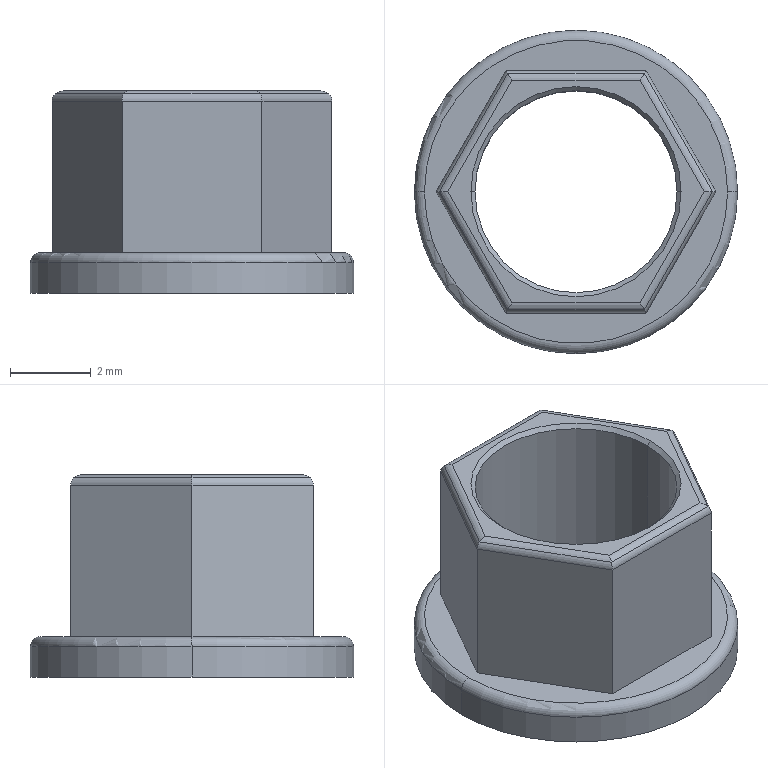Part | SolidWorks | features BaseBody 1 | 1 solid | 29 faces | box 8 x 8 x 5 mm | volume 76.113 mm3 | cylinder 16 | plane 9 | cone 2 | torus 2 | commonest cylinder face diameters 0.5 x12 5 x2 8 x2
STEP:
#1=CARTESIAN_POINT('',(-2.5,0.,4.9));
#2=VERTEX_POINT('',#1);
#3=CARTESIAN_POINT('',(2.5,0.,4.9));
#4=VERTEX_POINT('',#3);
#5=CARTESIAN_POINT('',(0.,0.,4.9));
#6=DIRECTION('',(0.,0.,-1.));
#7=DIRECTION('',(-1.,0.,0.));
#8=AXIS2_PLACEMENT_3D('',#5,#6,#7);
#9=CIRCLE('',#8,2.5);
#10=EDGE_CURVE('',#2,#4,#9,.T.);
#11=ORIENTED_EDGE('',*,*,#10,.T.);
#12=CARTESIAN_POINT('',(2.6,0.,5.));
#13=VERTEX_POINT('',#12);
#14=CARTESIAN_POINT('',(2.55,0.,4.95));
#15=DIRECTION('',(0.7071,0.,0.7071));
#16=VECTOR('',#15,1000.);
#17=LINE('',#14,#16);
#18=EDGE_CURVE('',#4,#13,#17,.T.);
#19=ORIENTED_EDGE('',*,*,#18,.T.);
#20=CARTESIAN_POINT('',(-2.6,0.,5.));
#21=VERTEX_POINT('',#20);
#22=CARTESIAN_POINT('',(0.,0.,5.));
#23=DIRECTION('',(0.,0.,1.));
#24=DIRECTION('',(-1.,0.,0.));
#25=AXIS2_PLACEMENT_3D('',#22,#23,#24);
#26=CIRCLE('',#25,2.6);
#27=EDGE_CURVE('',#13,#21,#26,.T.);
#28=ORIENTED_EDGE('',*,*,#27,.T.);
#29=CARTESIAN_POINT('',(-2.55,0.,4.95));
#30=DIRECTION('',(-0.7071,0.,0.7071));
#31=VECTOR('',#30,1000.);
#32=LINE('',#29,#31);
#33=EDGE_CURVE('',#2,#21,#32,.T.);
#34=ORIENTED_EDGE('',*,*,#33,.F.);
#35=EDGE_LOOP('',(#11,#19,#28,#34));
#36=FACE_OUTER_BOUND('',#35,.T.);
#37=CARTESIAN_POINT('',(0.,0.,4.95));
#38=DIRECTION('',(0.,0.,1.));
#39=DIRECTION('',(-1.,0.,0.));
#40=AXIS2_PLACEMENT_3D('',#37,#38,#39);
#41=CONICAL_SURFACE('',#40,2.55,0.7854);
#42=ADVANCED_FACE('',(#36),#41,.F.);
#43=CARTESIAN_POINT('',(2.5,0.,0.));
#44=VERTEX_POINT('',#43);
#45=CARTESIAN_POINT('',(-2.5,0.,0.));
#46=VERTEX_POINT('',#45);
#47=CARTESIAN_POINT('',(0.,0.,0.));
#48=DIRECTION('',(0.,0.,1.));
#49=DIRECTION('',(-1.,0.,0.));
#50=AXIS2_PLACEMENT_3D('',#47,#48,#49);
#51=CIRCLE('',#50,2.5);
#52=EDGE_CURVE('',#44,#46,#51,.T.);
#53=ORIENTED_EDGE('',*,*,#52,.F.);
#54=CARTESIAN_POINT('',(2.5,0.,5.));
#55=DIRECTION('',(0.,0.,1.));
#56=VECTOR('',#55,1000.);
#57=LINE('',#54,#56);
#58=EDGE_CURVE('',#44,#4,#57,.T.);
#59=ORIENTED_EDGE('',*,*,#58,.T.);
#60=ORIENTED_EDGE('',*,*,#10,.F.);
#61=CARTESIAN_POINT('',(-2.5,0.,5.));
#62=DIRECTION('',(0.,0.,1.));
#63=VECTOR('',#62,1000.);
#64=LINE('',#61,#63);
#65=EDGE_CURVE('',#46,#2,#64,.T.);
#66=ORIENTED_EDGE('',*,*,#65,.F.);
#67=EDGE_LOOP('',(#53,#59,#60,#66));
#68=FACE_OUTER_BOUND('',#67,.T.);
#69=CARTESIAN_POINT('',(0.,0.,5.));
#70=DIRECTION('',(0.,0.,1.));
#71=DIRECTION('',(-1.,0.,0.));
#72=AXIS2_PLACEMENT_3D('',#69,#70,#71);
#73=CYLINDRICAL_SURFACE('',#72,2.5);
#74=ADVANCED_FACE('',(#68),#73,.F.);
#75=CARTESIAN_POINT('',(4.,0.,0.75));
#76=VERTEX_POINT('',#75);
#77=CARTESIAN_POINT('',(-4.,0.,0.75));
#78=VERTEX_POINT('',#77);
#79=CARTESIAN_POINT('',(0.,0.,0.75));
#80=DIRECTION('',(0.,0.,1.));
#81=DIRECTION('',(-1.,0.,0.));
#82=AXIS2_PLACEMENT_3D('',#79,#80,#81);
#83=CIRCLE('',#82,4.);
#84=EDGE_CURVE('',#76,#78,#83,.T.);
#85=ORIENTED_EDGE('',*,*,#84,.T.);
#86=CARTESIAN_POINT('',(-3.75,0.,1.));
#87=VERTEX_POINT('',#86);
#88=CARTESIAN_POINT('',(-3.75,0.,0.75));
#89=DIRECTION('',(0.,1.,0.));
#90=DIRECTION('',(-1.,0.,0.));
#91=AXIS2_PLACEMENT_3D('',#88,#89,#90);
#92=CIRCLE('',#91,0.25);
#93=EDGE_CURVE('',#78,#87,#92,.T.);
#94=ORIENTED_EDGE('',*,*,#93,.T.);
#95=CARTESIAN_POINT('',(3.75,0.,1.));
#96=VERTEX_POINT('',#95);
#97=CARTESIAN_POINT('',(0.,0.,1.));
#98=DIRECTION('',(0.,0.,-1.));
#99=DIRECTION('',(-1.,0.,0.));
#100=AXIS2_PLACEMENT_3D('',#97,#98,#99);
#101=CIRCLE('',#100,3.75);
#102=EDGE_CURVE('',#87,#96,#101,.T.);
#103=ORIENTED_EDGE('',*,*,#102,.T.);
#104=CARTESIAN_POINT('',(3.75,0.,0.75));
#105=DIRECTION('',(0.,-1.,0.));
#106=DIRECTION('',(0.,0.,-1.));
#107=AXIS2_PLACEMENT_3D('',#104,#105,#106);
#108=CIRCLE('',#107,0.25);
#109=EDGE_CURVE('',#76,#96,#108,.T.);
#110=ORIENTED_EDGE('',*,*,#109,.F.);
#111=EDGE_LOOP('',(#85,#94,#103,#110));
#112=FACE_OUTER_BOUND('',#111,.T.);
#113=CARTESIAN_POINT('',(0.,0.,0.75));
#114=DIRECTION('',(0.,0.,1.));
#115=DIRECTION('',(1.,0.,0.));
#116=AXIS2_PLACEMENT_3D('',#113,#114,#115);
#117=TOROIDAL_SURFACE('',#116,3.75,0.25);
#118=ADVANCED_FACE('',(#112),#117,.T.);
#119=ORIENTED_EDGE('',*,*,#84,.F.);
#120=CARTESIAN_POINT('',(4.,0.,0.));
#121=VERTEX_POINT('',#120);
#122=CARTESIAN_POINT('',(4.,0.,0.));
#123=DIRECTION('',(0.,0.,-1.));
#124=VECTOR('',#123,1000.);
#125=LINE('',#122,#124);
#126=EDGE_CURVE('',#76,#121,#125,.T.);
#127=ORIENTED_EDGE('',*,*,#126,.T.);
#128=CARTESIAN_POINT('',(-4.,0.,0.));
#129=VERTEX_POINT('',#128);
#130=CARTESIAN_POINT('',(0.,0.,0.));
#131=DIRECTION('',(0.,0.,-1.));
#132=DIRECTION('',(-1.,0.,0.));
#133=AXIS2_PLACEMENT_3D('',#130,#131,#132);
#134=CIRCLE('',#133,4.);
#135=EDGE_CURVE('',#129,#121,#134,.T.);
#136=ORIENTED_EDGE('',*,*,#135,.F.);
#137=CARTESIAN_POINT('',(-4.,0.,0.));
#138=DIRECTION('',(0.,0.,-1.));
#139=VECTOR('',#138,1000.);
#140=LINE('',#137,#139);
#141=EDGE_CURVE('',#78,#129,#140,.T.);
#142=ORIENTED_EDGE('',*,*,#141,.F.);
#143=EDGE_LOOP('',(#119,#127,#136,#142));
#144=FACE_OUTER_BOUND('',#143,.T.);
#145=CARTESIAN_POINT('',(0.,0.,0.));
#146=DIRECTION('',(0.,0.,-1.));
#147=DIRECTION('',(-1.,0.,0.));
#148=AXIS2_PLACEMENT_3D('',#145,#146,#147);
#149=CYLINDRICAL_SURFACE('',#148,4.);
#150=ADVANCED_FACE('',(#144),#149,.T.);
#151=CARTESIAN_POINT('',(3.38,0.,4.927));
#152=VERTEX_POINT('',#151);
#153=CARTESIAN_POINT('',(3.464,0.,4.75));
#154=VERTEX_POINT('',#153);
#155=CARTESIAN_POINT('',(3.38,0.,4.927));
#156=CARTESIAN_POINT('',(3.434,0.,4.879));
#157=CARTESIAN_POINT('',(3.464,0.,4.817));
#158=CARTESIAN_POINT('',(3.464,0.,4.75));
#159=(BOUNDED_CURVE()B_SPLINE_CURVE(3,(#155,#156,#157,#158),.UNSPECIFIED.,.F.,.T.)B_SPLINE_CURVE_WITH_KNOTS((4,4),(5.498,6.283),.UNSPECIFIED.)CURVE()GEOMETRIC_REPRESENTATION_ITEM()RATIONAL_B_SPLINE_CURVE((1.,0.9493,0.9493,1.))REPRESENTATION_ITEM(''));
#160=EDGE_CURVE('',#152,#154,#159,.T.);
#161=ORIENTED_EDGE('',*,*,#160,.F.);
#162=CARTESIAN_POINT('',(1.69,-2.927,4.927));
#163=VERTEX_POINT('',#162);
#164=CARTESIAN_POINT('',(2.102,-2.213,4.927));
#165=DIRECTION('',(-0.5,-0.866,0.));
#166=VECTOR('',#165,1000.);
#167=LINE('',#164,#166);
#168=EDGE_CURVE('',#152,#163,#167,.T.);
#169=ORIENTED_EDGE('',*,*,#168,.T.);
#170=CARTESIAN_POINT('',(1.732,-3.,4.75));
#171=VERTEX_POINT('',#170);
#172=CARTESIAN_POINT('',(1.69,-2.927,4.927));
#173=CARTESIAN_POINT('',(1.717,-2.974,4.879));
#174=CARTESIAN_POINT('',(1.732,-3.,4.817));
#175=CARTESIAN_POINT('',(1.732,-3.,4.75));
#176=(BOUNDED_CURVE()B_SPLINE_CURVE(3,(#172,#173,#174,#175),.UNSPECIFIED.,.F.,.F.)B_SPLINE_CURVE_WITH_KNOTS((4,4),(5.498,6.283),.UNSPECIFIED.)CURVE()GEOMETRIC_REPRESENTATION_ITEM()RATIONAL_B_SPLINE_CURVE((1.,0.9493,0.9493,1.))REPRESENTATION_ITEM(''));
#177=EDGE_CURVE('',#163,#171,#176,.T.);
#178=ORIENTED_EDGE('',*,*,#177,.T.);
#179=CARTESIAN_POINT('',(2.165,-2.25,4.75));
#180=DIRECTION('',(0.5,0.866,0.));
#181=VECTOR('',#180,1000.);
#182=LINE('',#179,#181);
#183=EDGE_CURVE('',#171,#154,#182,.T.);
#184=ORIENTED_EDGE('',*,*,#183,.T.);
#185=EDGE_LOOP('',(#161,#169,#178,#184));
#186=FACE_OUTER_BOUND('',#185,.T.);
#187=CARTESIAN_POINT('',(1.949,-2.125,4.75));
#188=DIRECTION('',(-0.5,-0.866,0.));
#189=DIRECTION('',(0.6124,-0.3536,0.7071));
#190=AXIS2_PLACEMENT_3D('',#187,#188,#189);
#191=CYLINDRICAL_SURFACE('',#190,0.25);
#192=ADVANCED_FACE('',(#186),#191,.T.);
#193=ORIENTED_EDGE('',*,*,#177,.F.);
#194=CARTESIAN_POINT('',(-1.69,-2.927,4.927));
#195=VERTEX_POINT('',#194);
#196=CARTESIAN_POINT('',(-0.866,-2.927,4.927));
#197=DIRECTION('',(-1.,0.,0.));
#198=VECTOR('',#197,1000.);
#199=LINE('',#196,#198);
#200=EDGE_CURVE('',#163,#195,#199,.T.);
#201=ORIENTED_EDGE('',*,*,#200,.T.);
#202=CARTESIAN_POINT('',(-1.732,-3.,4.75));
#203=VERTEX_POINT('',#202);
#204=CARTESIAN_POINT('',(-1.69,-2.927,4.927));
#205=CARTESIAN_POINT('',(-1.717,-2.974,4.879));
#206=CARTESIAN_POINT('',(-1.732,-3.,4.817));
#207=CARTESIAN_POINT('',(-1.732,-3.,4.75));
#208=(BOUNDED_CURVE()B_SPLINE_CURVE(3,(#204,#205,#206,#207),.UNSPECIFIED.,.F.,.F.)B_SPLINE_CURVE_WITH_KNOTS((4,4),(5.498,6.283),.UNSPECIFIED.)CURVE()GEOMETRIC_REPRESENTATION_ITEM()RATIONAL_B_SPLINE_CURVE((1.,0.9493,0.9493,1.))REPRESENTATION_ITEM(''));
#209=EDGE_CURVE('',#195,#203,#208,.T.);
#210=ORIENTED_EDGE('',*,*,#209,.T.);
#211=CARTESIAN_POINT('',(-0.866,-3.,4.75));
#212=DIRECTION('',(1.,0.,0.));
#213=VECTOR('',#212,1000.);
#214=LINE('',#211,#213);
#215=EDGE_CURVE('',#203,#171,#214,.T.);
#216=ORIENTED_EDGE('',*,*,#215,.T.);
#217=EDGE_LOOP('',(#193,#201,#210,#216));
#218=FACE_OUTER_BOUND('',#217,.T.);
#219=CARTESIAN_POINT('',(-0.866,-2.75,4.75));
#220=DIRECTION('',(-1.,0.,0.));
#221=DIRECTION('',(0.,-0.7071,0.7071));
#222=AXIS2_PLACEMENT_3D('',#219,#220,#221);
#223=CYLINDRICAL_SURFACE('',#222,0.25);
#224=ADVANCED_FACE('',(#218),#223,.T.);
#225=ORIENTED_EDGE('',*,*,#209,.F.);
#226=CARTESIAN_POINT('',(-3.38,0.,4.927));
#227=VERTEX_POINT('',#226);
#228=CARTESIAN_POINT('',(-2.968,-0.7134,4.927));
#229=DIRECTION('',(-0.5,0.866,0.));
#230=VECTOR('',#229,1000.);
#231=LINE('',#228,#230);
#232=EDGE_CURVE('',#195,#227,#231,.T.);
#233=ORIENTED_EDGE('',*,*,#232,.T.);
#234=CARTESIAN_POINT('',(-3.464,0.,4.75));
#235=VERTEX_POINT('',#234);
#236=CARTESIAN_POINT('',(-3.38,0.,4.927));
#237=CARTESIAN_POINT('',(-3.434,0.,4.879));
#238=CARTESIAN_POINT('',(-3.464,0.,4.817));
#239=CARTESIAN_POINT('',(-3.464,0.,4.75));
#240=(BOUNDED_CURVE()B_SPLINE_CURVE(3,(#236,#237,#238,#239),.UNSPECIFIED.,.F.,.T.)B_SPLINE_CURVE_WITH_KNOTS((4,4),(5.498,6.283),.UNSPECIFIED.)CURVE()GEOMETRIC_REPRESENTATION_ITEM()RATIONAL_B_SPLINE_CURVE((1.,0.9493,0.9493,1.))REPRESENTATION_ITEM(''));
#241=EDGE_CURVE('',#227,#235,#240,.T.);
#242=ORIENTED_EDGE('',*,*,#241,.T.);
#243=CARTESIAN_POINT('',(-3.031,-0.75,4.75));
#244=DIRECTION('',(0.5,-0.866,0.));
#245=VECTOR('',#244,1000.);
#246=LINE('',#243,#245);
#247=EDGE_CURVE('',#235,#203,#246,.T.);
#248=ORIENTED_EDGE('',*,*,#247,.T.);
#249=EDGE_LOOP('',(#225,#233,#242,#248));
#250=FACE_OUTER_BOUND('',#249,.T.);
#251=CARTESIAN_POINT('',(-2.815,-0.625,4.75));
#252=DIRECTION('',(-0.5,0.866,0.));
#253=DIRECTION('',(-0.6124,-0.3536,0.7071));
#254=AXIS2_PLACEMENT_3D('',#251,#252,#253);
#255=CYLINDRICAL_SURFACE('',#254,0.25);
#256=ADVANCED_FACE('',(#250),#255,.T.);
#257=ORIENTED_EDGE('',*,*,#241,.F.);
#258=CARTESIAN_POINT('',(-1.69,2.927,4.927));
#259=VERTEX_POINT('',#258);
#260=CARTESIAN_POINT('',(-2.102,2.213,4.927));
#261=DIRECTION('',(0.5,0.866,0.));
#262=VECTOR('',#261,1000.);
#263=LINE('',#260,#262);
#264=EDGE_CURVE('',#227,#259,#263,.T.);
#265=ORIENTED_EDGE('',*,*,#264,.T.);
#266=CARTESIAN_POINT('',(-1.732,3.,4.75));
#267=VERTEX_POINT('',#266);
#268=CARTESIAN_POINT('',(-1.69,2.927,4.927));
#269=CARTESIAN_POINT('',(-1.717,2.974,4.879));
#270=CARTESIAN_POINT('',(-1.732,3.,4.817));
#271=CARTESIAN_POINT('',(-1.732,3.,4.75));
#272=(BOUNDED_CURVE()B_SPLINE_CURVE(3,(#268,#269,#270,#271),.UNSPECIFIED.,.F.,.T.)B_SPLINE_CURVE_WITH_KNOTS((4,4),(5.498,6.283),.UNSPECIFIED.)CURVE()GEOMETRIC_REPRESENTATION_ITEM()RATIONAL_B_SPLINE_CURVE((1.,0.9493,0.9493,1.))REPRESENTATION_ITEM(''));
#273=EDGE_CURVE('',#259,#267,#272,.T.);
#274=ORIENTED_EDGE('',*,*,#273,.T.);
#275=CARTESIAN_POINT('',(-2.165,2.25,4.75));
#276=DIRECTION('',(-0.5,-0.866,0.));
#277=VECTOR('',#276,1000.);
#278=LINE('',#275,#277);
#279=EDGE_CURVE('',#267,#235,#278,.T.);
#280=ORIENTED_EDGE('',*,*,#279,.T.);
#281=EDGE_LOOP('',(#257,#265,#274,#280));
#282=FACE_OUTER_BOUND('',#281,.T.);
#283=CARTESIAN_POINT('',(-1.949,2.125,4.75));
#284=DIRECTION('',(0.5,0.866,0.));
#285=DIRECTION('',(-0.6124,0.3536,0.7071));
#286=AXIS2_PLACEMENT_3D('',#283,#284,#285);
#287=CYLINDRICAL_SURFACE('',#286,0.25);
#288=ADVANCED_FACE('',(#282),#287,.T.);
#289=ORIENTED_EDGE('',*,*,#273,.F.);
#290=CARTESIAN_POINT('',(1.69,2.927,4.927));
#291=VERTEX_POINT('',#290);
#292=CARTESIAN_POINT('',(0.866,2.927,4.927));
#293=DIRECTION('',(1.,0.,0.));
#294=VECTOR('',#293,1000.);
#295=LINE('',#292,#294);
#296=EDGE_CURVE('',#259,#291,#295,.T.);
#297=ORIENTED_EDGE('',*,*,#296,.T.);
#298=CARTESIAN_POINT('',(1.732,3.,4.75));
#299=VERTEX_POINT('',#298);
#300=CARTESIAN_POINT('',(1.69,2.927,4.927));
#301=CARTESIAN_POINT('',(1.717,2.974,4.879));
#302=CARTESIAN_POINT('',(1.732,3.,4.817));
#303=CARTESIAN_POINT('',(1.732,3.,4.75));
#304=(BOUNDED_CURVE()B_SPLINE_CURVE(3,(#300,#301,#302,#303),.UNSPECIFIED.,.F.,.F.)B_SPLINE_CURVE_WITH_KNOTS((4,4),(5.498,6.283),.UNSPECIFIED.)CURVE()GEOMETRIC_REPRESENTATION_ITEM()RATIONAL_B_SPLINE_CURVE((1.,0.9493,0.9493,1.))REPRESENTATION_ITEM(''));
#305=EDGE_CURVE('',#291,#299,#304,.T.);
#306=ORIENTED_EDGE('',*,*,#305,.T.);
#307=CARTESIAN_POINT('',(0.866,3.,4.75));
#308=DIRECTION('',(-1.,0.,0.));
#309=VECTOR('',#308,1000.);
#310=LINE('',#307,#309);
#311=EDGE_CURVE('',#299,#267,#310,.T.);
#312=ORIENTED_EDGE('',*,*,#311,.T.);
#313=EDGE_LOOP('',(#289,#297,#306,#312));
#314=FACE_OUTER_BOUND('',#313,.T.);
#315=CARTESIAN_POINT('',(0.866,2.75,4.75));
#316=DIRECTION('',(1.,0.,0.));
#317=DIRECTION('',(0.,0.7071,0.7071));
#318=AXIS2_PLACEMENT_3D('',#315,#316,#317);
#319=CYLINDRICAL_SURFACE('',#318,0.25);
#320=ADVANCED_FACE('',(#314),#319,.T.);
#321=ORIENTED_EDGE('',*,*,#305,.F.);
#322=CARTESIAN_POINT('',(2.968,0.7134,4.927));
#323=DIRECTION('',(0.5,-0.866,0.));
#324=VECTOR('',#323,1000.);
#325=LINE('',#322,#324);
#326=EDGE_CURVE('',#291,#152,#325,.T.);
#327=ORIENTED_EDGE('',*,*,#326,.T.);
#328=ORIENTED_EDGE('',*,*,#160,.T.);
#329=CARTESIAN_POINT('',(3.031,0.75,4.75));
#330=DIRECTION('',(-0.5,0.866,0.));
#331=VECTOR('',#330,1000.);
#332=LINE('',#329,#331);
#333=EDGE_CURVE('',#154,#299,#332,.T.);
#334=ORIENTED_EDGE('',*,*,#333,.T.);
#335=EDGE_LOOP('',(#321,#327,#328,#334));
#336=FACE_OUTER_BOUND('',#335,.T.);
#337=CARTESIAN_POINT('',(2.815,0.625,4.75));
#338=DIRECTION('',(0.5,-0.866,0.));
#339=DIRECTION('',(0.6124,0.3536,0.7071));
#340=AXIS2_PLACEMENT_3D('',#337,#338,#339);
#341=CYLINDRICAL_SURFACE('',#340,0.25);
#342=ADVANCED_FACE('',(#336),#341,.T.);
#343=CARTESIAN_POINT('',(0.,0.,5.));
#344=DIRECTION('',(0.,0.,1.));
#345=DIRECTION('',(-1.,0.,0.));
#346=AXIS2_PLACEMENT_3D('',#343,#344,#345);
#347=CIRCLE('',#346,2.6);
#348=EDGE_CURVE('',#21,#13,#347,.T.);
#349=ORIENTED_EDGE('',*,*,#348,.F.);
#350=ORIENTED_EDGE('',*,*,#27,.F.);
#351=EDGE_LOOP('',(#349,#350));
#352=FACE_BOUND('',#351,.T.);
#353=CARTESIAN_POINT('',(3.175,0.,5.));
#354=VERTEX_POINT('',#353);
#355=CARTESIAN_POINT('',(1.588,-2.75,5.));
#356=VERTEX_POINT('',#355);
#357=CARTESIAN_POINT('',(1.949,-2.125,5.));
#358=DIRECTION('',(-0.5,-0.866,0.));
#359=VECTOR('',#358,1000.);
#360=LINE('',#357,#359);
#361=EDGE_CURVE('',#354,#356,#360,.T.);
#362=ORIENTED_EDGE('',*,*,#361,.F.);
#363=CARTESIAN_POINT('',(1.588,2.75,5.));
#364=VERTEX_POINT('',#363);
#365=CARTESIAN_POINT('',(2.815,0.625,5.));
#366=DIRECTION('',(0.5,-0.866,0.));
#367=VECTOR('',#366,1000.);
#368=LINE('',#365,#367);
#369=EDGE_CURVE('',#364,#354,#368,.T.);
#370=ORIENTED_EDGE('',*,*,#369,.F.);
#371=CARTESIAN_POINT('',(-1.588,2.75,5.));
#372=VERTEX_POINT('',#371);
#373=CARTESIAN_POINT('',(0.866,2.75,5.));
#374=DIRECTION('',(1.,0.,0.));
#375=VECTOR('',#374,1000.);
#376=LINE('',#373,#375);
#377=EDGE_CURVE('',#372,#364,#376,.T.);
#378=ORIENTED_EDGE('',*,*,#377,.F.);
#379=CARTESIAN_POINT('',(-3.175,0.,5.));
#380=VERTEX_POINT('',#379);
#381=CARTESIAN_POINT('',(-1.949,2.125,5.));
#382=DIRECTION('',(0.5,0.866,0.));
#383=VECTOR('',#382,1000.);
#384=LINE('',#381,#383);
#385=EDGE_CURVE('',#380,#372,#384,.T.);
#386=ORIENTED_EDGE('',*,*,#385,.F.);
#387=CARTESIAN_POINT('',(-1.588,-2.75,5.));
#388=VERTEX_POINT('',#387);
#389=CARTESIAN_POINT('',(-2.815,-0.625,5.));
#390=DIRECTION('',(-0.5,0.866,0.));
#391=VECTOR('',#390,1000.);
#392=LINE('',#389,#391);
#393=EDGE_CURVE('',#388,#380,#392,.T.);
#394=ORIENTED_EDGE('',*,*,#393,.F.);
#395=CARTESIAN_POINT('',(-0.866,-2.75,5.));
#396=DIRECTION('',(-1.,0.,0.));
#397=VECTOR('',#396,1000.);
#398=LINE('',#395,#397);
#399=EDGE_CURVE('',#356,#388,#398,.T.);
#400=ORIENTED_EDGE('',*,*,#399,.F.);
#401=EDGE_LOOP('',(#362,#370,#378,#386,#394,#400));
#402=FACE_OUTER_BOUND('',#401,.T.);
#403=CARTESIAN_POINT('',(0.,0.,5.));
#404=DIRECTION('',(0.,0.,1.));
#405=DIRECTION('',(1.,0.,0.));
#406=AXIS2_PLACEMENT_3D('',#403,#404,#405);
#407=PLANE('',#406);
#408=ADVANCED_FACE('',(#352,#402),#407,.T.);
#409=CARTESIAN_POINT('',(-1.732,-3.,1.));
#410=VERTEX_POINT('',#409);
#411=CARTESIAN_POINT('',(-3.464,0.,1.));
#412=VERTEX_POINT('',#411);
#413=CARTESIAN_POINT('',(-3.031,-0.75,1.));
#414=DIRECTION('',(-0.5,0.866,0.));
#415=VECTOR('',#414,1000.);
#416=LINE('',#413,#415);
#417=EDGE_CURVE('',#410,#412,#416,.T.);
#418=ORIENTED_EDGE('',*,*,#417,.T.);
#419=CARTESIAN_POINT('',(-1.732,3.,1.));
#420=VERTEX_POINT('',#419);
#421=CARTESIAN_POINT('',(-2.165,2.25,1.));
#422=DIRECTION('',(0.5,0.866,0.));
#423=VECTOR('',#422,1000.);
#424=LINE('',#421,#423);
#425=EDGE_CURVE('',#412,#420,#424,.T.);
#426=ORIENTED_EDGE('',*,*,#425,.T.);
#427=CARTESIAN_POINT('',(1.732,3.,1.));
#428=VERTEX_POINT('',#427);
#429=CARTESIAN_POINT('',(0.866,3.,1.));
#430=DIRECTION('',(1.,0.,0.));
#431=VECTOR('',#430,1000.);
#432=LINE('',#429,#431);
#433=EDGE_CURVE('',#420,#428,#432,.T.);
#434=ORIENTED_EDGE('',*,*,#433,.T.);
#435=CARTESIAN_POINT('',(3.464,0.,1.));
#436=VERTEX_POINT('',#435);
#437=CARTESIAN_POINT('',(3.031,0.75,1.));
#438=DIRECTION('',(0.5,-0.866,0.));
#439=VECTOR('',#438,1000.);
#440=LINE('',#437,#439);
#441=EDGE_CURVE('',#428,#436,#440,.T.);
#442=ORIENTED_EDGE('',*,*,#441,.T.);
#443=CARTESIAN_POINT('',(1.732,-3.,1.));
#444=VERTEX_POINT('',#443);
#445=CARTESIAN_POINT('',(2.165,-2.25,1.));
#446=DIRECTION('',(-0.5,-0.866,0.));
#447=VECTOR('',#446,1000.);
#448=LINE('',#445,#447);
#449=EDGE_CURVE('',#436,#444,#448,.T.);
#450=ORIENTED_EDGE('',*,*,#449,.T.);
#451=CARTESIAN_POINT('',(-0.866,-3.,1.));
#452=DIRECTION('',(-1.,0.,0.));
#453=VECTOR('',#452,1000.);
#454=LINE('',#451,#453);
#455=EDGE_CURVE('',#444,#410,#454,.T.);
#456=ORIENTED_EDGE('',*,*,#455,.T.);
#457=EDGE_LOOP('',(#418,#426,#434,#442,#450,#456));
#458=FACE_BOUND('',#457,.T.);
#459=CARTESIAN_POINT('',(0.,0.,1.));
#460=DIRECTION('',(0.,0.,-1.));
#461=DIRECTION('',(-1.,0.,0.));
#462=AXIS2_PLACEMENT_3D('',#459,#460,#461);
#463=CIRCLE('',#462,3.75);
#464=EDGE_CURVE('',#96,#87,#463,.T.);
#465=ORIENTED_EDGE('',*,*,#464,.F.);
#466=ORIENTED_EDGE('',*,*,#102,.F.);
#467=EDGE_LOOP('',(#465,#466));
#468=FACE_OUTER_BOUND('',#467,.T.);
#469=CARTESIAN_POINT('',(0.,0.,1.));
#470=DIRECTION('',(0.,0.,1.));
#471=DIRECTION('',(1.,0.,0.));
#472=AXIS2_PLACEMENT_3D('',#469,#470,#471);
#473=PLANE('',#472);
#474=ADVANCED_FACE('',(#458,#468),#473,.T.);
#475=ORIENTED_EDGE('',*,*,#311,.F.);
#476=CARTESIAN_POINT('',(1.732,3.,1.));
#477=DIRECTION('',(0.,0.,1.));
#478=VECTOR('',#477,1000.);
#479=LINE('',#476,#478);
#480=EDGE_CURVE('',#428,#299,#479,.T.);
#481=ORIENTED_EDGE('',*,*,#480,.F.);
#482=ORIENTED_EDGE('',*,*,#433,.F.);
#483=CARTESIAN_POINT('',(-1.732,3.,1.));
#484=DIRECTION('',(0.,0.,1.));
#485=VECTOR('',#484,1000.);
#486=LINE('',#483,#485);
#487=EDGE_CURVE('',#420,#267,#486,.T.);
#488=ORIENTED_EDGE('',*,*,#487,.T.);
#489=EDGE_LOOP('',(#475,#481,#482,#488));
#490=FACE_OUTER_BOUND('',#489,.T.);
#491=CARTESIAN_POINT('',(1.732,3.,1.));
#492=DIRECTION('',(0.,1.,0.));
#493=DIRECTION('',(1.,0.,0.));
#494=AXIS2_PLACEMENT_3D('',#491,#492,#493);
#495=PLANE('',#494);
#496=ADVANCED_FACE('',(#490),#495,.T.);
#497=ORIENTED_EDGE('',*,*,#333,.F.);
#498=CARTESIAN_POINT('',(3.464,0.,1.));
#499=DIRECTION('',(0.,0.,1.));
#500=VECTOR('',#499,1000.);
#501=LINE('',#498,#500);
#502=EDGE_CURVE('',#436,#154,#501,.T.);
#503=ORIENTED_EDGE('',*,*,#502,.F.);
#504=ORIENTED_EDGE('',*,*,#441,.F.);
#505=ORIENTED_EDGE('',*,*,#480,.T.);
#506=EDGE_LOOP('',(#497,#503,#504,#505));
#507=FACE_OUTER_BOUND('',#506,.T.);
#508=CARTESIAN_POINT('',(3.464,0.,1.));
#509=DIRECTION('',(0.866,0.5,0.));
#510=DIRECTION('',(0.,0.,-1.));
#511=AXIS2_PLACEMENT_3D('',#508,#509,#510);
#512=PLANE('',#511);
#513=ADVANCED_FACE('',(#507),#512,.T.);
#514=ORIENTED_EDGE('',*,*,#183,.F.);
#515=CARTESIAN_POINT('',(1.732,-3.,1.));
#516=DIRECTION('',(0.,0.,1.));
#517=VECTOR('',#516,1000.);
#518=LINE('',#515,#517);
#519=EDGE_CURVE('',#444,#171,#518,.T.);
#520=ORIENTED_EDGE('',*,*,#519,.F.);
#521=ORIENTED_EDGE('',*,*,#449,.F.);
#522=ORIENTED_EDGE('',*,*,#502,.T.);
#523=EDGE_LOOP('',(#514,#520,#521,#522));
#524=FACE_OUTER_BOUND('',#523,.T.);
#525=CARTESIAN_POINT('',(1.732,-3.,1.));
#526=DIRECTION('',(0.866,-0.5,0.));
#527=DIRECTION('',(0.,0.,-1.));
#528=AXIS2_PLACEMENT_3D('',#525,#526,#527);
#529=PLANE('',#528);
#530=ADVANCED_FACE('',(#524),#529,.T.);
#531=ORIENTED_EDGE('',*,*,#247,.F.);
#532=CARTESIAN_POINT('',(-3.464,0.,1.));
#533=DIRECTION('',(0.,0.,1.));
#534=VECTOR('',#533,1000.);
#535=LINE('',#532,#534);
#536=EDGE_CURVE('',#412,#235,#535,.T.);
#537=ORIENTED_EDGE('',*,*,#536,.F.);
#538=ORIENTED_EDGE('',*,*,#417,.F.);
#539=CARTESIAN_POINT('',(-1.732,-3.,1.));
#540=DIRECTION('',(0.,0.,1.));
#541=VECTOR('',#540,1000.);
#542=LINE('',#539,#541);
#543=EDGE_CURVE('',#410,#203,#542,.T.);
#544=ORIENTED_EDGE('',*,*,#543,.T.);
#545=EDGE_LOOP('',(#531,#537,#538,#544));
#546=FACE_OUTER_BOUND('',#545,.T.);
#547=CARTESIAN_POINT('',(-3.464,0.,1.));
#548=DIRECTION('',(-0.866,-0.5,0.));
#549=DIRECTION('',(-0.5,0.866,0.));
#550=AXIS2_PLACEMENT_3D('',#547,#548,#549);
#551=PLANE('',#550);
#552=ADVANCED_FACE('',(#546),#551,.T.);
#553=ORIENTED_EDGE('',*,*,#279,.F.);
#554=ORIENTED_EDGE('',*,*,#487,.F.);
#555=ORIENTED_EDGE('',*,*,#425,.F.);
#556=ORIENTED_EDGE('',*,*,#536,.T.);
#557=EDGE_LOOP('',(#553,#554,#555,#556));
#558=FACE_OUTER_BOUND('',#557,.T.);
#559=CARTESIAN_POINT('',(-1.732,3.,1.));
#560=DIRECTION('',(-0.866,0.5,0.));
#561=DIRECTION('',(0.,0.,1.));
#562=AXIS2_PLACEMENT_3D('',#559,#560,#561);
#563=PLANE('',#562);
#564=ADVANCED_FACE('',(#558),#563,.T.);
#565=ORIENTED_EDGE('',*,*,#215,.F.);
#566=ORIENTED_EDGE('',*,*,#543,.F.);
#567=ORIENTED_EDGE('',*,*,#455,.F.);
#568=ORIENTED_EDGE('',*,*,#519,.T.);
#569=EDGE_LOOP('',(#565,#566,#567,#568));
#570=FACE_OUTER_BOUND('',#569,.T.);
#571=CARTESIAN_POINT('',(-1.732,-3.,1.));
#572=DIRECTION('',(0.,-1.,0.));
#573=DIRECTION('',(-1.,0.,0.));
#574=AXIS2_PLACEMENT_3D('',#571,#572,#573);
#575=PLANE('',#574);
#576=ADVANCED_FACE('',(#570),#575,.T.);
#577=CARTESIAN_POINT('',(0.,0.,0.));
#578=DIRECTION('',(0.,0.,1.));
#579=DIRECTION('',(-1.,0.,0.));
#580=AXIS2_PLACEMENT_3D('',#577,#578,#579);
#581=CIRCLE('',#580,2.5);
#582=EDGE_CURVE('',#46,#44,#581,.T.);
#583=ORIENTED_EDGE('',*,*,#582,.T.);
#584=ORIENTED_EDGE('',*,*,#52,.T.);
#585=EDGE_LOOP('',(#583,#584));
#586=FACE_BOUND('',#585,.T.);
#587=ORIENTED_EDGE('',*,*,#135,.T.);
#588=CARTESIAN_POINT('',(0.,0.,0.));
#589=DIRECTION('',(0.,0.,-1.));
#590=DIRECTION('',(-1.,0.,0.));
#591=AXIS2_PLACEMENT_3D('',#588,#589,#590);
#592=CIRCLE('',#591,4.);
#593=EDGE_CURVE('',#121,#129,#592,.T.);
#594=ORIENTED_EDGE('',*,*,#593,.T.);
#595=EDGE_LOOP('',(#587,#594));
#596=FACE_OUTER_BOUND('',#595,.T.);
#597=CARTESIAN_POINT('',(0.,0.,0.));
#598=DIRECTION('',(0.,0.,1.));
#599=DIRECTION('',(1.,0.,0.));
#600=AXIS2_PLACEMENT_3D('',#597,#598,#599);
#601=PLANE('',#600);
#602=ADVANCED_FACE('',(#586,#596),#601,.F.);
#603=ORIENTED_EDGE('',*,*,#326,.F.);
#604=CARTESIAN_POINT('',(1.588,2.75,5.));
#605=CARTESIAN_POINT('',(1.627,2.817,5.));
#606=CARTESIAN_POINT('',(1.662,2.879,4.974));
#607=CARTESIAN_POINT('',(1.69,2.927,4.927));
#608=(BOUNDED_CURVE()B_SPLINE_CURVE(3,(#604,#605,#606,#607),.UNSPECIFIED.,.F.,.F.)B_SPLINE_CURVE_WITH_KNOTS((4,4),(4.712,5.498),.UNSPECIFIED.)CURVE()GEOMETRIC_REPRESENTATION_ITEM()RATIONAL_B_SPLINE_CURVE((1.,0.9493,0.9493,1.))REPRESENTATION_ITEM(''));
#609=EDGE_CURVE('',#364,#291,#608,.T.);
#610=ORIENTED_EDGE('',*,*,#609,.F.);
#611=ORIENTED_EDGE('',*,*,#369,.T.);
#612=CARTESIAN_POINT('',(3.175,0.,5.));
#613=CARTESIAN_POINT('',(3.253,0.,5.));
#614=CARTESIAN_POINT('',(3.325,0.,4.974));
#615=CARTESIAN_POINT('',(3.38,0.,4.927));
#616=(BOUNDED_CURVE()B_SPLINE_CURVE(3,(#612,#613,#614,#615),.UNSPECIFIED.,.F.,.T.)B_SPLINE_CURVE_WITH_KNOTS((4,4),(4.712,5.498),.UNSPECIFIED.)CURVE()GEOMETRIC_REPRESENTATION_ITEM()RATIONAL_B_SPLINE_CURVE((1.,0.9493,0.9493,1.))REPRESENTATION_ITEM(''));
#617=EDGE_CURVE('',#354,#152,#616,.T.);
#618=ORIENTED_EDGE('',*,*,#617,.T.);
#619=EDGE_LOOP('',(#603,#610,#611,#618));
#620=FACE_OUTER_BOUND('',#619,.T.);
#621=CARTESIAN_POINT('',(2.815,0.625,4.75));
#622=DIRECTION('',(0.5,-0.866,0.));
#623=DIRECTION('',(0.6124,0.3536,0.7071));
#624=AXIS2_PLACEMENT_3D('',#621,#622,#623);
#625=CYLINDRICAL_SURFACE('',#624,0.25);
#626=ADVANCED_FACE('',(#620),#625,.T.);
#627=ORIENTED_EDGE('',*,*,#296,.F.);
#628=CARTESIAN_POINT('',(-1.588,2.75,5.));
#629=CARTESIAN_POINT('',(-1.627,2.817,5.));
#630=CARTESIAN_POINT('',(-1.662,2.879,4.974));
#631=CARTESIAN_POINT('',(-1.69,2.927,4.927));
#632=(BOUNDED_CURVE()B_SPLINE_CURVE(3,(#628,#629,#630,#631),.UNSPECIFIED.,.F.,.T.)B_SPLINE_CURVE_WITH_KNOTS((4,4),(4.712,5.498),.UNSPECIFIED.)CURVE()GEOMETRIC_REPRESENTATION_ITEM()RATIONAL_B_SPLINE_CURVE((1.,0.9493,0.9493,1.))REPRESENTATION_ITEM(''));
#633=EDGE_CURVE('',#372,#259,#632,.T.);
#634=ORIENTED_EDGE('',*,*,#633,.F.);
#635=ORIENTED_EDGE('',*,*,#377,.T.);
#636=ORIENTED_EDGE('',*,*,#609,.T.);
#637=EDGE_LOOP('',(#627,#634,#635,#636));
#638=FACE_OUTER_BOUND('',#637,.T.);
#639=CARTESIAN_POINT('',(0.866,2.75,4.75));
#640=DIRECTION('',(1.,0.,0.));
#641=DIRECTION('',(0.,0.7071,0.7071));
#642=AXIS2_PLACEMENT_3D('',#639,#640,#641);
#643=CYLINDRICAL_SURFACE('',#642,0.25);
#644=ADVANCED_FACE('',(#638),#643,.T.);
#645=ORIENTED_EDGE('',*,*,#264,.F.);
#646=CARTESIAN_POINT('',(-3.175,0.,5.));
#647=CARTESIAN_POINT('',(-3.253,0.,5.));
#648=CARTESIAN_POINT('',(-3.325,0.,4.974));
#649=CARTESIAN_POINT('',(-3.38,0.,4.927));
#650=(BOUNDED_CURVE()B_SPLINE_CURVE(3,(#646,#647,#648,#649),.UNSPECIFIED.,.F.,.F.)B_SPLINE_CURVE_WITH_KNOTS((4,4),(4.712,5.498),.UNSPECIFIED.)CURVE()GEOMETRIC_REPRESENTATION_ITEM()RATIONAL_B_SPLINE_CURVE((1.,0.9493,0.9493,1.))REPRESENTATION_ITEM(''));
#651=EDGE_CURVE('',#380,#227,#650,.T.);
#652=ORIENTED_EDGE('',*,*,#651,.F.);
#653=ORIENTED_EDGE('',*,*,#385,.T.);
#654=ORIENTED_EDGE('',*,*,#633,.T.);
#655=EDGE_LOOP('',(#645,#652,#653,#654));
#656=FACE_OUTER_BOUND('',#655,.T.);
#657=CARTESIAN_POINT('',(-1.949,2.125,4.75));
#658=DIRECTION('',(0.5,0.866,0.));
#659=DIRECTION('',(-0.6124,0.3536,0.7071));
#660=AXIS2_PLACEMENT_3D('',#657,#658,#659);
#661=CYLINDRICAL_SURFACE('',#660,0.25);
#662=ADVANCED_FACE('',(#656),#661,.T.);
#663=ORIENTED_EDGE('',*,*,#232,.F.);
#664=CARTESIAN_POINT('',(-1.588,-2.75,5.));
#665=CARTESIAN_POINT('',(-1.627,-2.817,5.));
#666=CARTESIAN_POINT('',(-1.662,-2.879,4.974));
#667=CARTESIAN_POINT('',(-1.69,-2.927,4.927));
#668=(BOUNDED_CURVE()B_SPLINE_CURVE(3,(#664,#665,#666,#667),.UNSPECIFIED.,.F.,.F.)B_SPLINE_CURVE_WITH_KNOTS((4,4),(4.712,5.498),.UNSPECIFIED.)CURVE()GEOMETRIC_REPRESENTATION_ITEM()RATIONAL_B_SPLINE_CURVE((1.,0.9493,0.9493,1.))REPRESENTATION_ITEM(''));
#669=EDGE_CURVE('',#388,#195,#668,.T.);
#670=ORIENTED_EDGE('',*,*,#669,.F.);
#671=ORIENTED_EDGE('',*,*,#393,.T.);
#672=ORIENTED_EDGE('',*,*,#651,.T.);
#673=EDGE_LOOP('',(#663,#670,#671,#672));
#674=FACE_OUTER_BOUND('',#673,.T.);
#675=CARTESIAN_POINT('',(-2.815,-0.625,4.75));
#676=DIRECTION('',(-0.5,0.866,0.));
#677=DIRECTION('',(-0.6124,-0.3536,0.7071));
#678=AXIS2_PLACEMENT_3D('',#675,#676,#677);
#679=CYLINDRICAL_SURFACE('',#678,0.25);
#680=ADVANCED_FACE('',(#674),#679,.T.);
#681=ORIENTED_EDGE('',*,*,#200,.F.);
#682=CARTESIAN_POINT('',(1.588,-2.75,5.));
#683=CARTESIAN_POINT('',(1.627,-2.817,5.));
#684=CARTESIAN_POINT('',(1.662,-2.879,4.974));
#685=CARTESIAN_POINT('',(1.69,-2.927,4.927));
#686=(BOUNDED_CURVE()B_SPLINE_CURVE(3,(#682,#683,#684,#685),.UNSPECIFIED.,.F.,.F.)B_SPLINE_CURVE_WITH_KNOTS((4,4),(4.712,5.498),.UNSPECIFIED.)CURVE()GEOMETRIC_REPRESENTATION_ITEM()RATIONAL_B_SPLINE_CURVE((1.,0.9493,0.9493,1.))REPRESENTATION_ITEM(''));
#687=EDGE_CURVE('',#356,#163,#686,.T.);
#688=ORIENTED_EDGE('',*,*,#687,.F.);
#689=ORIENTED_EDGE('',*,*,#399,.T.);
#690=ORIENTED_EDGE('',*,*,#669,.T.);
#691=EDGE_LOOP('',(#681,#688,#689,#690));
#692=FACE_OUTER_BOUND('',#691,.T.);
#693=CARTESIAN_POINT('',(-0.866,-2.75,4.75));
#694=DIRECTION('',(-1.,0.,0.));
#695=DIRECTION('',(0.,-0.7071,0.7071));
#696=AXIS2_PLACEMENT_3D('',#693,#694,#695);
#697=CYLINDRICAL_SURFACE('',#696,0.25);
#698=ADVANCED_FACE('',(#692),#697,.T.);
#699=ORIENTED_EDGE('',*,*,#168,.F.);
#700=ORIENTED_EDGE('',*,*,#617,.F.);
#701=ORIENTED_EDGE('',*,*,#361,.T.);
#702=ORIENTED_EDGE('',*,*,#687,.T.);
#703=EDGE_LOOP('',(#699,#700,#701,#702));
#704=FACE_OUTER_BOUND('',#703,.T.);
#705=CARTESIAN_POINT('',(1.949,-2.125,4.75));
#706=DIRECTION('',(-0.5,-0.866,0.));
#707=DIRECTION('',(0.6124,-0.3536,0.7071));
#708=AXIS2_PLACEMENT_3D('',#705,#706,#707);
#709=CYLINDRICAL_SURFACE('',#708,0.25);
#710=ADVANCED_FACE('',(#704),#709,.T.);
#711=ORIENTED_EDGE('',*,*,#126,.F.);
#712=CARTESIAN_POINT('',(0.,0.,0.75));
#713=DIRECTION('',(0.,0.,1.));
#714=DIRECTION('',(-1.,0.,0.));
#715=AXIS2_PLACEMENT_3D('',#712,#713,#714);
#716=CIRCLE('',#715,4.);
#717=EDGE_CURVE('',#78,#76,#716,.T.);
#718=ORIENTED_EDGE('',*,*,#717,.F.);
#719=ORIENTED_EDGE('',*,*,#141,.T.);
#720=ORIENTED_EDGE('',*,*,#593,.F.);
#721=EDGE_LOOP('',(#711,#718,#719,#720));
#722=FACE_OUTER_BOUND('',#721,.T.);
#723=CARTESIAN_POINT('',(0.,0.,0.));
#724=DIRECTION('',(0.,0.,-1.));
#725=DIRECTION('',(-1.,0.,0.));
#726=AXIS2_PLACEMENT_3D('',#723,#724,#725);
#727=CYLINDRICAL_SURFACE('',#726,4.);
#728=ADVANCED_FACE('',(#722),#727,.T.);
#729=ORIENTED_EDGE('',*,*,#93,.F.);
#730=ORIENTED_EDGE('',*,*,#717,.T.);
#731=ORIENTED_EDGE('',*,*,#109,.T.);
#732=ORIENTED_EDGE('',*,*,#464,.T.);
#733=EDGE_LOOP('',(#729,#730,#731,#732));
#734=FACE_OUTER_BOUND('',#733,.T.);
#735=CARTESIAN_POINT('',(0.,0.,0.75));
#736=DIRECTION('',(0.,0.,1.));
#737=DIRECTION('',(1.,0.,0.));
#738=AXIS2_PLACEMENT_3D('',#735,#736,#737);
#739=TOROIDAL_SURFACE('',#738,3.75,0.25);
#740=ADVANCED_FACE('',(#734),#739,.T.);
#741=ORIENTED_EDGE('',*,*,#58,.F.);
#742=ORIENTED_EDGE('',*,*,#582,.F.);
#743=ORIENTED_EDGE('',*,*,#65,.T.);
#744=CARTESIAN_POINT('',(0.,0.,4.9));
#745=DIRECTION('',(0.,0.,-1.));
#746=DIRECTION('',(-1.,0.,0.));
#747=AXIS2_PLACEMENT_3D('',#744,#745,#746);
#748=CIRCLE('',#747,2.5);
#749=EDGE_CURVE('',#4,#2,#748,.T.);
#750=ORIENTED_EDGE('',*,*,#749,.F.);
#751=EDGE_LOOP('',(#741,#742,#743,#750));
#752=FACE_OUTER_BOUND('',#751,.T.);
#753=CARTESIAN_POINT('',(0.,0.,5.));
#754=DIRECTION('',(0.,0.,1.));
#755=DIRECTION('',(-1.,0.,0.));
#756=AXIS2_PLACEMENT_3D('',#753,#754,#755);
#757=CYLINDRICAL_SURFACE('',#756,2.5);
#758=ADVANCED_FACE('',(#752),#757,.F.);
#759=ORIENTED_EDGE('',*,*,#18,.F.);
#760=ORIENTED_EDGE('',*,*,#749,.T.);
#761=ORIENTED_EDGE('',*,*,#33,.T.);
#762=ORIENTED_EDGE('',*,*,#348,.T.);
#763=EDGE_LOOP('',(#759,#760,#761,#762));
#764=FACE_OUTER_BOUND('',#763,.T.);
#765=CARTESIAN_POINT('',(0.,0.,4.95));
#766=DIRECTION('',(0.,0.,1.));
#767=DIRECTION('',(-1.,0.,0.));
#768=AXIS2_PLACEMENT_3D('',#765,#766,#767);
#769=CONICAL_SURFACE('',#768,2.55,0.7854);
#770=ADVANCED_FACE('',(#764),#769,.F.);
#771=CLOSED_SHELL('',(#42,#74,#118,#150,#192,#224,#256,#288,#320,#342,#408,#474,#496,#513,#530,#552,#564,#576,#602,#626,#644,#662,#680,#698,#710,#728,#740,#758,#770));
#772=MANIFOLD_SOLID_BREP('',#771);
#773=CARTESIAN_POINT('',(0.,0.,0.));
#774=DIRECTION('',(0.,0.,1.));
#775=DIRECTION('',(1.,0.,0.));
#776=AXIS2_PLACEMENT_3D('',#773,#774,#775);
#777=(LENGTH_UNIT()NAMED_UNIT(*)SI_UNIT(.MILLI.,.METRE.));
#778=UNCERTAINTY_MEASURE_WITH_UNIT(LENGTH_MEASURE(0.00001),#777,'','');
#779=(NAMED_UNIT(*)PLANE_ANGLE_UNIT()SI_UNIT($,.RADIAN.));
#780=(NAMED_UNIT(*)SI_UNIT($,.STERADIAN.)SOLID_ANGLE_UNIT());
#781=(GEOMETRIC_REPRESENTATION_CONTEXT(3)GLOBAL_UNCERTAINTY_ASSIGNED_CONTEXT((#778))GLOBAL_UNIT_ASSIGNED_CONTEXT((#777,#779,#780))REPRESENTATION_CONTEXT('',''));
#782=ADVANCED_BREP_SHAPE_REPRESENTATION('',(#772,#776),#781);